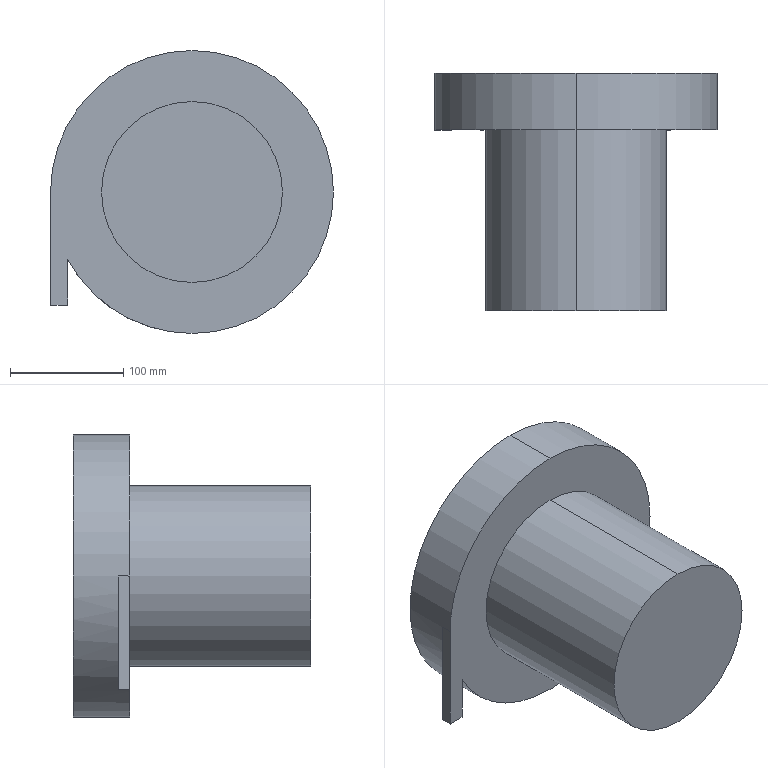Part | STEP file | Vibration plate3 | 1 solid | 11 faces | box 250 x 210 x 250 mm | volume 5680348 mm3 | plane 7 | cylinder 4 | commonest cylinder face diameters 160 x2 250 x2
STEP:
#1=CARTESIAN_POINT('',(0.,0.,0.));
#2=DIRECTION('',(0.,0.,1.));
#3=DIRECTION('',(1.,0.,0.));
#4=AXIS2_PLACEMENT_3D('',#1,#2,#3);
#5=CARTESIAN_POINT('',(0.,210.,125.));
#6=VERTEX_POINT('',#5);
#7=CARTESIAN_POINT('',(0.,210.,-125.));
#8=VERTEX_POINT('',#7);
#9=CARTESIAN_POINT('',(0.,210.,0.));
#10=DIRECTION('',(0.,1.,0.));
#11=DIRECTION('',(0.,0.,1.));
#12=AXIS2_PLACEMENT_3D('',#9,#10,#11);
#13=CIRCLE('',#12,125.);
#14=CARTESIAN_POINT('',(0.,210.,0.));
#15=DIRECTION('',(0.,-1.,0.));
#16=DIRECTION('',(0.,0.,-1.));
#17=AXIS2_PLACEMENT_3D('',#14,#15,#16);
#18=CYLINDRICAL_SURFACE('',#17,125.);
#19=CARTESIAN_POINT('',(3.142,0.));
#20=DIRECTION('',(-1.,0.));
#21=VECTOR('',#20,1.);
#22=LINE('',#19,#21);
#23=(GEOMETRIC_REPRESENTATION_CONTEXT(2)PARAMETRIC_REPRESENTATION_CONTEXT()REPRESENTATION_CONTEXT('',''));
#24=DEFINITIONAL_REPRESENTATION('',(#22),#23);
#25=PCURVE('',#18,#24);
#26=CARTESIAN_POINT('',(0.,210.,0.));
#27=DIRECTION('',(0.,1.,0.));
#28=DIRECTION('',(0.,0.,1.));
#29=AXIS2_PLACEMENT_3D('',#26,#27,#28);
#30=PLANE('',#29);
#31=CARTESIAN_POINT('',(0.,0.));
#32=DIRECTION('',(1.,0.));
#33=AXIS2_PLACEMENT_2D('',#31,#32);
#34=CIRCLE('',#33,125.);
#35=(GEOMETRIC_REPRESENTATION_CONTEXT(2)PARAMETRIC_REPRESENTATION_CONTEXT()REPRESENTATION_CONTEXT('',''));
#36=DEFINITIONAL_REPRESENTATION('',(#34),#35);
#37=PCURVE('',#30,#36);
#38=SURFACE_CURVE('',#13,(#25,#37),.PCURVE_S1.);
#39=EDGE_CURVE('',#6,#8,#38,.T.);
#40=ORIENTED_EDGE('',*,*,#39,.F.);
#41=CARTESIAN_POINT('',(0.,160.,125.));
#42=VERTEX_POINT('',#41);
#43=CARTESIAN_POINT('',(0.,210.,125.));
#44=DIRECTION('',(0.,-1.,0.));
#45=VECTOR('',#44,1.);
#46=LINE('',#43,#45);
#47=CARTESIAN_POINT('',(3.142,0.));
#48=DIRECTION('',(0.,1.));
#49=VECTOR('',#48,1.);
#50=LINE('',#47,#49);
#51=(GEOMETRIC_REPRESENTATION_CONTEXT(2)PARAMETRIC_REPRESENTATION_CONTEXT()REPRESENTATION_CONTEXT('',''));
#52=DEFINITIONAL_REPRESENTATION('',(#50),#51);
#53=PCURVE('',#18,#52);
#54=CARTESIAN_POINT('',(0.,210.,0.));
#55=DIRECTION('',(0.,-1.,0.));
#56=DIRECTION('',(0.,0.,-1.));
#57=AXIS2_PLACEMENT_3D('',#54,#55,#56);
#58=CYLINDRICAL_SURFACE('',#57,125.);
#59=CARTESIAN_POINT('',(3.142,0.));
#60=DIRECTION('',(0.,1.));
#61=VECTOR('',#60,1.);
#62=LINE('',#59,#61);
#63=(GEOMETRIC_REPRESENTATION_CONTEXT(2)PARAMETRIC_REPRESENTATION_CONTEXT()REPRESENTATION_CONTEXT('',''));
#64=DEFINITIONAL_REPRESENTATION('',(#62),#63);
#65=PCURVE('',#58,#64);
#66=SURFACE_CURVE('',#46,(#53,#65),.PCURVE_S1.);
#67=EDGE_CURVE('',#6,#42,#66,.T.);
#68=ORIENTED_EDGE('',*,*,#67,.T.);
#69=CARTESIAN_POINT('',(0.,160.,-125.));
#70=VERTEX_POINT('',#69);
#71=CARTESIAN_POINT('',(0.,160.,0.));
#72=DIRECTION('',(0.,1.,0.));
#73=DIRECTION('',(0.,0.,1.));
#74=AXIS2_PLACEMENT_3D('',#71,#72,#73);
#75=CIRCLE('',#74,125.);
#76=CARTESIAN_POINT('',(3.142,50.));
#77=DIRECTION('',(-1.,0.));
#78=VECTOR('',#77,1.);
#79=LINE('',#76,#78);
#80=(GEOMETRIC_REPRESENTATION_CONTEXT(2)PARAMETRIC_REPRESENTATION_CONTEXT()REPRESENTATION_CONTEXT('',''));
#81=DEFINITIONAL_REPRESENTATION('',(#79),#80);
#82=PCURVE('',#18,#81);
#83=CARTESIAN_POINT('',(0.,160.,0.));
#84=DIRECTION('',(0.,1.,0.));
#85=DIRECTION('',(0.,0.,1.));
#86=AXIS2_PLACEMENT_3D('',#83,#84,#85);
#87=PLANE('',#86);
#88=CARTESIAN_POINT('',(0.,0.));
#89=DIRECTION('',(1.,0.));
#90=AXIS2_PLACEMENT_2D('',#88,#89);
#91=CIRCLE('',#90,125.);
#92=(GEOMETRIC_REPRESENTATION_CONTEXT(2)PARAMETRIC_REPRESENTATION_CONTEXT()REPRESENTATION_CONTEXT('',''));
#93=DEFINITIONAL_REPRESENTATION('',(#91),#92);
#94=PCURVE('',#87,#93);
#95=SURFACE_CURVE('',#75,(#82,#94),.PCURVE_S1.);
#96=EDGE_CURVE('',#42,#70,#95,.T.);
#97=ORIENTED_EDGE('',*,*,#96,.T.);
#98=CARTESIAN_POINT('',(0.,210.,-125.));
#99=DIRECTION('',(0.,-1.,0.));
#100=VECTOR('',#99,1.);
#101=LINE('',#98,#100);
#102=CARTESIAN_POINT('',(0.,0.));
#103=DIRECTION('',(0.,1.));
#104=VECTOR('',#103,1.);
#105=LINE('',#102,#104);
#106=(GEOMETRIC_REPRESENTATION_CONTEXT(2)PARAMETRIC_REPRESENTATION_CONTEXT()REPRESENTATION_CONTEXT('',''));
#107=DEFINITIONAL_REPRESENTATION('',(#105),#106);
#108=PCURVE('',#18,#107);
#109=CARTESIAN_POINT('',(6.283,0.));
#110=DIRECTION('',(0.,1.));
#111=VECTOR('',#110,1.);
#112=LINE('',#109,#111);
#113=(GEOMETRIC_REPRESENTATION_CONTEXT(2)PARAMETRIC_REPRESENTATION_CONTEXT()REPRESENTATION_CONTEXT('',''));
#114=DEFINITIONAL_REPRESENTATION('',(#112),#113);
#115=PCURVE('',#58,#114);
#116=SURFACE_CURVE('',#101,(#108,#115),.PCURVE_S1.);
#117=EDGE_CURVE('',#8,#70,#116,.T.);
#118=ORIENTED_EDGE('',*,*,#117,.F.);
#119=EDGE_LOOP('',(#40,#68,#97,#118));
#120=FACE_BOUND('',#119,.T.);
#121=ADVANCED_FACE('',(#120),#18,.T.);
#122=CARTESIAN_POINT('',(0.,160.,80.));
#123=VERTEX_POINT('',#122);
#124=CARTESIAN_POINT('',(0.,160.,-80.));
#125=VERTEX_POINT('',#124);
#126=CARTESIAN_POINT('',(0.,160.,0.));
#127=DIRECTION('',(0.,1.,0.));
#128=DIRECTION('',(0.,0.,1.));
#129=AXIS2_PLACEMENT_3D('',#126,#127,#128);
#130=CIRCLE('',#129,80.);
#131=CARTESIAN_POINT('',(0.,160.,0.));
#132=DIRECTION('',(0.,-1.,0.));
#133=DIRECTION('',(0.,0.,-1.));
#134=AXIS2_PLACEMENT_3D('',#131,#132,#133);
#135=CYLINDRICAL_SURFACE('',#134,80.);
#136=CARTESIAN_POINT('',(3.142,0.));
#137=DIRECTION('',(-1.,0.));
#138=VECTOR('',#137,1.);
#139=LINE('',#136,#138);
#140=(GEOMETRIC_REPRESENTATION_CONTEXT(2)PARAMETRIC_REPRESENTATION_CONTEXT()REPRESENTATION_CONTEXT('',''));
#141=DEFINITIONAL_REPRESENTATION('',(#139),#140);
#142=PCURVE('',#135,#141);
#143=CARTESIAN_POINT('',(0.,0.));
#144=DIRECTION('',(1.,0.));
#145=AXIS2_PLACEMENT_2D('',#143,#144);
#146=CIRCLE('',#145,80.);
#147=(GEOMETRIC_REPRESENTATION_CONTEXT(2)PARAMETRIC_REPRESENTATION_CONTEXT()REPRESENTATION_CONTEXT('',''));
#148=DEFINITIONAL_REPRESENTATION('',(#146),#147);
#149=PCURVE('',#87,#148);
#150=SURFACE_CURVE('',#130,(#142,#149),.PCURVE_S1.);
#151=EDGE_CURVE('',#123,#125,#150,.T.);
#152=ORIENTED_EDGE('',*,*,#151,.F.);
#153=CARTESIAN_POINT('',(0.,0.,80.));
#154=VERTEX_POINT('',#153);
#155=CARTESIAN_POINT('',(0.,160.,80.));
#156=DIRECTION('',(0.,-1.,0.));
#157=VECTOR('',#156,1.);
#158=LINE('',#155,#157);
#159=CARTESIAN_POINT('',(3.142,0.));
#160=DIRECTION('',(0.,1.));
#161=VECTOR('',#160,1.);
#162=LINE('',#159,#161);
#163=(GEOMETRIC_REPRESENTATION_CONTEXT(2)PARAMETRIC_REPRESENTATION_CONTEXT()REPRESENTATION_CONTEXT('',''));
#164=DEFINITIONAL_REPRESENTATION('',(#162),#163);
#165=PCURVE('',#135,#164);
#166=CARTESIAN_POINT('',(0.,160.,0.));
#167=DIRECTION('',(0.,-1.,0.));
#168=DIRECTION('',(0.,0.,-1.));
#169=AXIS2_PLACEMENT_3D('',#166,#167,#168);
#170=CYLINDRICAL_SURFACE('',#169,80.);
#171=CARTESIAN_POINT('',(3.142,0.));
#172=DIRECTION('',(0.,1.));
#173=VECTOR('',#172,1.);
#174=LINE('',#171,#173);
#175=(GEOMETRIC_REPRESENTATION_CONTEXT(2)PARAMETRIC_REPRESENTATION_CONTEXT()REPRESENTATION_CONTEXT('',''));
#176=DEFINITIONAL_REPRESENTATION('',(#174),#175);
#177=PCURVE('',#170,#176);
#178=SURFACE_CURVE('',#158,(#165,#177),.PCURVE_S1.);
#179=EDGE_CURVE('',#123,#154,#178,.T.);
#180=ORIENTED_EDGE('',*,*,#179,.T.);
#181=CARTESIAN_POINT('',(0.,0.,-80.));
#182=VERTEX_POINT('',#181);
#183=CARTESIAN_POINT('',(0.,0.,0.));
#184=DIRECTION('',(0.,1.,0.));
#185=DIRECTION('',(0.,0.,1.));
#186=AXIS2_PLACEMENT_3D('',#183,#184,#185);
#187=CIRCLE('',#186,80.);
#188=CARTESIAN_POINT('',(3.142,160.));
#189=DIRECTION('',(-1.,0.));
#190=VECTOR('',#189,1.);
#191=LINE('',#188,#190);
#192=(GEOMETRIC_REPRESENTATION_CONTEXT(2)PARAMETRIC_REPRESENTATION_CONTEXT()REPRESENTATION_CONTEXT('',''));
#193=DEFINITIONAL_REPRESENTATION('',(#191),#192);
#194=PCURVE('',#135,#193);
#195=CARTESIAN_POINT('',(0.,0.,0.));
#196=DIRECTION('',(0.,1.,0.));
#197=DIRECTION('',(0.,0.,1.));
#198=AXIS2_PLACEMENT_3D('',#195,#196,#197);
#199=PLANE('',#198);
#200=CARTESIAN_POINT('',(0.,0.));
#201=DIRECTION('',(1.,0.));
#202=AXIS2_PLACEMENT_2D('',#200,#201);
#203=CIRCLE('',#202,80.);
#204=(GEOMETRIC_REPRESENTATION_CONTEXT(2)PARAMETRIC_REPRESENTATION_CONTEXT()REPRESENTATION_CONTEXT('',''));
#205=DEFINITIONAL_REPRESENTATION('',(#203),#204);
#206=PCURVE('',#199,#205);
#207=SURFACE_CURVE('',#187,(#194,#206),.PCURVE_S1.);
#208=EDGE_CURVE('',#154,#182,#207,.T.);
#209=ORIENTED_EDGE('',*,*,#208,.T.);
#210=CARTESIAN_POINT('',(0.,160.,-80.));
#211=DIRECTION('',(0.,-1.,0.));
#212=VECTOR('',#211,1.);
#213=LINE('',#210,#212);
#214=CARTESIAN_POINT('',(0.,0.));
#215=DIRECTION('',(0.,1.));
#216=VECTOR('',#215,1.);
#217=LINE('',#214,#216);
#218=(GEOMETRIC_REPRESENTATION_CONTEXT(2)PARAMETRIC_REPRESENTATION_CONTEXT()REPRESENTATION_CONTEXT('',''));
#219=DEFINITIONAL_REPRESENTATION('',(#217),#218);
#220=PCURVE('',#135,#219);
#221=CARTESIAN_POINT('',(6.283,0.));
#222=DIRECTION('',(0.,1.));
#223=VECTOR('',#222,1.);
#224=LINE('',#221,#223);
#225=(GEOMETRIC_REPRESENTATION_CONTEXT(2)PARAMETRIC_REPRESENTATION_CONTEXT()REPRESENTATION_CONTEXT('',''));
#226=DEFINITIONAL_REPRESENTATION('',(#224),#225);
#227=PCURVE('',#170,#226);
#228=SURFACE_CURVE('',#213,(#220,#227),.PCURVE_S1.);
#229=EDGE_CURVE('',#125,#182,#228,.T.);
#230=ORIENTED_EDGE('',*,*,#229,.F.);
#231=EDGE_LOOP('',(#152,#180,#209,#230));
#232=FACE_BOUND('',#231,.T.);
#233=ADVANCED_FACE('',(#232),#135,.T.);
#234=ORIENTED_EDGE('',*,*,#179,.F.);
#235=CARTESIAN_POINT('',(0.,160.,0.));
#236=DIRECTION('',(0.,1.,0.));
#237=DIRECTION('',(0.,0.,1.));
#238=AXIS2_PLACEMENT_3D('',#235,#236,#237);
#239=CIRCLE('',#238,80.);
#240=CARTESIAN_POINT('',(9.425,0.));
#241=DIRECTION('',(-1.,0.));
#242=VECTOR('',#241,1.);
#243=LINE('',#240,#242);
#244=(GEOMETRIC_REPRESENTATION_CONTEXT(2)PARAMETRIC_REPRESENTATION_CONTEXT()REPRESENTATION_CONTEXT('',''));
#245=DEFINITIONAL_REPRESENTATION('',(#243),#244);
#246=PCURVE('',#170,#245);
#247=CARTESIAN_POINT('',(0.,0.));
#248=DIRECTION('',(1.,0.));
#249=AXIS2_PLACEMENT_2D('',#247,#248);
#250=CIRCLE('',#249,80.);
#251=(GEOMETRIC_REPRESENTATION_CONTEXT(2)PARAMETRIC_REPRESENTATION_CONTEXT()REPRESENTATION_CONTEXT('',''));
#252=DEFINITIONAL_REPRESENTATION('',(#250),#251);
#253=PCURVE('',#87,#252);
#254=SURFACE_CURVE('',#239,(#246,#253),.PCURVE_S1.);
#255=EDGE_CURVE('',#125,#123,#254,.T.);
#256=ORIENTED_EDGE('',*,*,#255,.F.);
#257=ORIENTED_EDGE('',*,*,#229,.T.);
#258=CARTESIAN_POINT('',(0.,0.,0.));
#259=DIRECTION('',(0.,1.,0.));
#260=DIRECTION('',(0.,0.,1.));
#261=AXIS2_PLACEMENT_3D('',#258,#259,#260);
#262=CIRCLE('',#261,80.);
#263=CARTESIAN_POINT('',(9.425,160.));
#264=DIRECTION('',(-1.,0.));
#265=VECTOR('',#264,1.);
#266=LINE('',#263,#265);
#267=(GEOMETRIC_REPRESENTATION_CONTEXT(2)PARAMETRIC_REPRESENTATION_CONTEXT()REPRESENTATION_CONTEXT('',''));
#268=DEFINITIONAL_REPRESENTATION('',(#266),#267);
#269=PCURVE('',#170,#268);
#270=CARTESIAN_POINT('',(0.,0.));
#271=DIRECTION('',(1.,0.));
#272=AXIS2_PLACEMENT_2D('',#270,#271);
#273=CIRCLE('',#272,80.);
#274=(GEOMETRIC_REPRESENTATION_CONTEXT(2)PARAMETRIC_REPRESENTATION_CONTEXT()REPRESENTATION_CONTEXT('',''));
#275=DEFINITIONAL_REPRESENTATION('',(#273),#274);
#276=PCURVE('',#199,#275);
#277=SURFACE_CURVE('',#262,(#269,#276),.PCURVE_S1.);
#278=EDGE_CURVE('',#182,#154,#277,.T.);
#279=ORIENTED_EDGE('',*,*,#278,.T.);
#280=EDGE_LOOP('',(#234,#256,#257,#279));
#281=FACE_BOUND('',#280,.T.);
#282=ADVANCED_FACE('',(#281),#170,.T.);
#283=ORIENTED_EDGE('',*,*,#278,.F.);
#284=ORIENTED_EDGE('',*,*,#208,.F.);
#285=EDGE_LOOP('',(#283,#284));
#286=FACE_BOUND('',#285,.T.);
#287=ADVANCED_FACE('',(#286),#199,.F.);
#288=CARTESIAN_POINT('',(-125.,160.,0.));
#289=VERTEX_POINT('',#288);
#290=CARTESIAN_POINT('',(0.,160.,0.));
#291=DIRECTION('',(0.,1.,0.));
#292=DIRECTION('',(0.,0.,1.));
#293=AXIS2_PLACEMENT_3D('',#290,#291,#292);
#294=CIRCLE('',#293,125.);
#295=CARTESIAN_POINT('',(0.,0.));
#296=DIRECTION('',(1.,0.));
#297=AXIS2_PLACEMENT_2D('',#295,#296);
#298=CIRCLE('',#297,125.);
#299=(GEOMETRIC_REPRESENTATION_CONTEXT(2)PARAMETRIC_REPRESENTATION_CONTEXT()REPRESENTATION_CONTEXT('',''));
#300=DEFINITIONAL_REPRESENTATION('',(#298),#299);
#301=PCURVE('',#87,#300);
#302=CARTESIAN_POINT('',(9.425,50.));
#303=DIRECTION('',(-1.,0.));
#304=VECTOR('',#303,1.);
#305=LINE('',#302,#304);
#306=(GEOMETRIC_REPRESENTATION_CONTEXT(2)PARAMETRIC_REPRESENTATION_CONTEXT()REPRESENTATION_CONTEXT('',''));
#307=DEFINITIONAL_REPRESENTATION('',(#305),#306);
#308=PCURVE('',#58,#307);
#309=SURFACE_CURVE('',#294,(#301,#308),.PCURVE_S1.);
#310=EDGE_CURVE('',#289,#42,#309,.T.);
#311=ORIENTED_EDGE('',*,*,#310,.F.);
#312=CARTESIAN_POINT('',(-125.,160.,-100.));
#313=VERTEX_POINT('',#312);
#314=CARTESIAN_POINT('',(-125.,160.,0.));
#315=DIRECTION('',(0.,0.,-1.));
#316=VECTOR('',#315,1.);
#317=LINE('',#314,#316);
#318=CARTESIAN_POINT('',(0.,-125.));
#319=DIRECTION('',(-1.,0.));
#320=VECTOR('',#319,1.);
#321=LINE('',#318,#320);
#322=(GEOMETRIC_REPRESENTATION_CONTEXT(2)PARAMETRIC_REPRESENTATION_CONTEXT()REPRESENTATION_CONTEXT('',''));
#323=DEFINITIONAL_REPRESENTATION('',(#321),#322);
#324=PCURVE('',#87,#323);
#325=CARTESIAN_POINT('',(-125.,170.,0.));
#326=DIRECTION('',(-1.,0.,0.));
#327=DIRECTION('',(0.,0.,1.));
#328=AXIS2_PLACEMENT_3D('',#325,#326,#327);
#329=PLANE('',#328);
#330=CARTESIAN_POINT('',(0.,-10.));
#331=DIRECTION('',(-1.,0.));
#332=VECTOR('',#331,1.);
#333=LINE('',#330,#332);
#334=(GEOMETRIC_REPRESENTATION_CONTEXT(2)PARAMETRIC_REPRESENTATION_CONTEXT()REPRESENTATION_CONTEXT('',''));
#335=DEFINITIONAL_REPRESENTATION('',(#333),#334);
#336=PCURVE('',#329,#335);
#337=SURFACE_CURVE('',#317,(#324,#336),.PCURVE_S1.);
#338=EDGE_CURVE('',#289,#313,#337,.T.);
#339=ORIENTED_EDGE('',*,*,#338,.T.);
#340=CARTESIAN_POINT('',(-110.,160.,-100.));
#341=VERTEX_POINT('',#340);
#342=CARTESIAN_POINT('',(-125.,160.,-100.));
#343=DIRECTION('',(1.,0.,0.));
#344=VECTOR('',#343,1.);
#345=LINE('',#342,#344);
#346=CARTESIAN_POINT('',(-100.,-125.));
#347=DIRECTION('',(0.,1.));
#348=VECTOR('',#347,1.);
#349=LINE('',#346,#348);
#350=(GEOMETRIC_REPRESENTATION_CONTEXT(2)PARAMETRIC_REPRESENTATION_CONTEXT()REPRESENTATION_CONTEXT('',''));
#351=DEFINITIONAL_REPRESENTATION('',(#349),#350);
#352=PCURVE('',#87,#351);
#353=CARTESIAN_POINT('',(-125.,170.,-100.));
#354=DIRECTION('',(0.,0.,-1.));
#355=DIRECTION('',(-1.,0.,0.));
#356=AXIS2_PLACEMENT_3D('',#353,#354,#355);
#357=PLANE('',#356);
#358=CARTESIAN_POINT('',(0.,-10.));
#359=DIRECTION('',(-1.,0.));
#360=VECTOR('',#359,1.);
#361=LINE('',#358,#360);
#362=(GEOMETRIC_REPRESENTATION_CONTEXT(2)PARAMETRIC_REPRESENTATION_CONTEXT()REPRESENTATION_CONTEXT('',''));
#363=DEFINITIONAL_REPRESENTATION('',(#361),#362);
#364=PCURVE('',#357,#363);
#365=SURFACE_CURVE('',#345,(#352,#364),.PCURVE_S1.);
#366=EDGE_CURVE('',#313,#341,#365,.T.);
#367=ORIENTED_EDGE('',*,*,#366,.T.);
#368=CARTESIAN_POINT('',(-110.,160.,-59.372));
#369=VERTEX_POINT('',#368);
#370=CARTESIAN_POINT('',(-110.,160.,0.));
#371=DIRECTION('',(0.,0.,1.));
#372=VECTOR('',#371,1.);
#373=LINE('',#370,#372);
#374=CARTESIAN_POINT('',(0.,-110.));
#375=DIRECTION('',(1.,0.));
#376=VECTOR('',#375,1.);
#377=LINE('',#374,#376);
#378=(GEOMETRIC_REPRESENTATION_CONTEXT(2)PARAMETRIC_REPRESENTATION_CONTEXT()REPRESENTATION_CONTEXT('',''));
#379=DEFINITIONAL_REPRESENTATION('',(#377),#378);
#380=PCURVE('',#87,#379);
#381=CARTESIAN_POINT('',(-110.,170.,0.));
#382=DIRECTION('',(1.,0.,0.));
#383=DIRECTION('',(0.,0.,-1.));
#384=AXIS2_PLACEMENT_3D('',#381,#382,#383);
#385=PLANE('',#384);
#386=CARTESIAN_POINT('',(0.,-10.));
#387=DIRECTION('',(-1.,0.));
#388=VECTOR('',#387,1.);
#389=LINE('',#386,#388);
#390=(GEOMETRIC_REPRESENTATION_CONTEXT(2)PARAMETRIC_REPRESENTATION_CONTEXT()REPRESENTATION_CONTEXT('',''));
#391=DEFINITIONAL_REPRESENTATION('',(#389),#390);
#392=PCURVE('',#385,#391);
#393=SURFACE_CURVE('',#373,(#380,#392),.PCURVE_S1.);
#394=EDGE_CURVE('',#341,#369,#393,.T.);
#395=ORIENTED_EDGE('',*,*,#394,.T.);
#396=CARTESIAN_POINT('',(0.,160.,0.));
#397=DIRECTION('',(0.,1.,0.));
#398=DIRECTION('',(0.,0.,1.));
#399=AXIS2_PLACEMENT_3D('',#396,#397,#398);
#400=CIRCLE('',#399,125.);
#401=CARTESIAN_POINT('',(0.,0.));
#402=DIRECTION('',(1.,0.));
#403=AXIS2_PLACEMENT_2D('',#401,#402);
#404=CIRCLE('',#403,125.);
#405=(GEOMETRIC_REPRESENTATION_CONTEXT(2)PARAMETRIC_REPRESENTATION_CONTEXT()REPRESENTATION_CONTEXT('',''));
#406=DEFINITIONAL_REPRESENTATION('',(#404),#405);
#407=PCURVE('',#87,#406);
#408=CARTESIAN_POINT('',(9.425,50.));
#409=DIRECTION('',(-1.,0.));
#410=VECTOR('',#409,1.);
#411=LINE('',#408,#410);
#412=(GEOMETRIC_REPRESENTATION_CONTEXT(2)PARAMETRIC_REPRESENTATION_CONTEXT()REPRESENTATION_CONTEXT('',''));
#413=DEFINITIONAL_REPRESENTATION('',(#411),#412);
#414=PCURVE('',#58,#413);
#415=SURFACE_CURVE('',#400,(#407,#414),.PCURVE_S1.);
#416=EDGE_CURVE('',#70,#369,#415,.T.);
#417=ORIENTED_EDGE('',*,*,#416,.F.);
#418=ORIENTED_EDGE('',*,*,#96,.F.);
#419=EDGE_LOOP('',(#311,#339,#367,#395,#417,#418));
#420=FACE_BOUND('',#419,.T.);
#421=ORIENTED_EDGE('',*,*,#255,.T.);
#422=ORIENTED_EDGE('',*,*,#151,.T.);
#423=EDGE_LOOP('',(#421,#422));
#424=FACE_BOUND('',#423,.T.);
#425=ADVANCED_FACE('',(#420,#424),#87,.F.);
#426=ORIENTED_EDGE('',*,*,#67,.F.);
#427=CARTESIAN_POINT('',(0.,210.,0.));
#428=DIRECTION('',(0.,1.,0.));
#429=DIRECTION('',(0.,0.,1.));
#430=AXIS2_PLACEMENT_3D('',#427,#428,#429);
#431=CIRCLE('',#430,125.);
#432=CARTESIAN_POINT('',(9.425,0.));
#433=DIRECTION('',(-1.,0.));
#434=VECTOR('',#433,1.);
#435=LINE('',#432,#434);
#436=(GEOMETRIC_REPRESENTATION_CONTEXT(2)PARAMETRIC_REPRESENTATION_CONTEXT()REPRESENTATION_CONTEXT('',''));
#437=DEFINITIONAL_REPRESENTATION('',(#435),#436);
#438=PCURVE('',#58,#437);
#439=CARTESIAN_POINT('',(0.,0.));
#440=DIRECTION('',(1.,0.));
#441=AXIS2_PLACEMENT_2D('',#439,#440);
#442=CIRCLE('',#441,125.);
#443=(GEOMETRIC_REPRESENTATION_CONTEXT(2)PARAMETRIC_REPRESENTATION_CONTEXT()REPRESENTATION_CONTEXT('',''));
#444=DEFINITIONAL_REPRESENTATION('',(#442),#443);
#445=PCURVE('',#30,#444);
#446=SURFACE_CURVE('',#431,(#438,#445),.PCURVE_S1.);
#447=EDGE_CURVE('',#8,#6,#446,.T.);
#448=ORIENTED_EDGE('',*,*,#447,.F.);
#449=ORIENTED_EDGE('',*,*,#117,.T.);
#450=ORIENTED_EDGE('',*,*,#416,.T.);
#451=CARTESIAN_POINT('',(-110.,170.,-59.372));
#452=VERTEX_POINT('',#451);
#453=CARTESIAN_POINT('',(-110.,210.,-59.372));
#454=DIRECTION('',(0.,1.,0.));
#455=VECTOR('',#454,1.);
#456=LINE('',#453,#455);
#457=CARTESIAN_POINT('',(5.207,0.));
#458=DIRECTION('',(0.,-1.));
#459=VECTOR('',#458,1.);
#460=LINE('',#457,#459);
#461=(GEOMETRIC_REPRESENTATION_CONTEXT(2)PARAMETRIC_REPRESENTATION_CONTEXT()REPRESENTATION_CONTEXT('',''));
#462=DEFINITIONAL_REPRESENTATION('',(#460),#461);
#463=PCURVE('',#58,#462);
#464=CARTESIAN_POINT('',(59.372,40.));
#465=DIRECTION('',(0.,1.));
#466=VECTOR('',#465,1.);
#467=LINE('',#464,#466);
#468=(GEOMETRIC_REPRESENTATION_CONTEXT(2)PARAMETRIC_REPRESENTATION_CONTEXT()REPRESENTATION_CONTEXT('',''));
#469=DEFINITIONAL_REPRESENTATION('',(#467),#468);
#470=PCURVE('',#385,#469);
#471=SURFACE_CURVE('',#456,(#463,#470),.PCURVE_S1.);
#472=EDGE_CURVE('',#369,#452,#471,.T.);
#473=ORIENTED_EDGE('',*,*,#472,.T.);
#474=CARTESIAN_POINT('',(-125.,170.,0.));
#475=VERTEX_POINT('',#474);
#476=CARTESIAN_POINT('',(0.,170.,0.));
#477=DIRECTION('',(0.,-1.,0.));
#478=DIRECTION('',(0.,0.,-1.));
#479=AXIS2_PLACEMENT_3D('',#476,#477,#478);
#480=CIRCLE('',#479,125.);
#481=CARTESIAN_POINT('',(0.,40.));
#482=DIRECTION('',(1.,0.));
#483=VECTOR('',#482,1.);
#484=LINE('',#481,#483);
#485=(GEOMETRIC_REPRESENTATION_CONTEXT(2)PARAMETRIC_REPRESENTATION_CONTEXT()REPRESENTATION_CONTEXT('',''));
#486=DEFINITIONAL_REPRESENTATION('',(#484),#485);
#487=PCURVE('',#58,#486);
#488=CARTESIAN_POINT('',(0.,170.,0.));
#489=DIRECTION('',(0.,-1.,0.));
#490=DIRECTION('',(0.,0.,-1.));
#491=AXIS2_PLACEMENT_3D('',#488,#489,#490);
#492=PLANE('',#491);
#493=CARTESIAN_POINT('',(0.,0.));
#494=DIRECTION('',(1.,0.));
#495=AXIS2_PLACEMENT_2D('',#493,#494);
#496=CIRCLE('',#495,125.);
#497=(GEOMETRIC_REPRESENTATION_CONTEXT(2)PARAMETRIC_REPRESENTATION_CONTEXT()REPRESENTATION_CONTEXT('',''));
#498=DEFINITIONAL_REPRESENTATION('',(#496),#497);
#499=PCURVE('',#492,#498);
#500=SURFACE_CURVE('',#480,(#487,#499),.PCURVE_S1.);
#501=EDGE_CURVE('',#475,#452,#500,.T.);
#502=ORIENTED_EDGE('',*,*,#501,.F.);
#503=CARTESIAN_POINT('',(-125.,170.,0.));
#504=DIRECTION('',(0.,-1.,0.));
#505=VECTOR('',#504,1.);
#506=LINE('',#503,#505);
#507=CARTESIAN_POINT('',(4.712,40.));
#508=DIRECTION('',(0.,1.));
#509=VECTOR('',#508,1.);
#510=LINE('',#507,#509);
#511=(GEOMETRIC_REPRESENTATION_CONTEXT(2)PARAMETRIC_REPRESENTATION_CONTEXT()REPRESENTATION_CONTEXT('',''));
#512=DEFINITIONAL_REPRESENTATION('',(#510),#511);
#513=PCURVE('',#58,#512);
#514=CARTESIAN_POINT('',(0.,0.));
#515=DIRECTION('',(0.,-1.));
#516=VECTOR('',#515,1.);
#517=LINE('',#514,#516);
#518=(GEOMETRIC_REPRESENTATION_CONTEXT(2)PARAMETRIC_REPRESENTATION_CONTEXT()REPRESENTATION_CONTEXT('',''));
#519=DEFINITIONAL_REPRESENTATION('',(#517),#518);
#520=PCURVE('',#329,#519);
#521=SURFACE_CURVE('',#506,(#513,#520),.PCURVE_S1.);
#522=EDGE_CURVE('',#475,#289,#521,.T.);
#523=ORIENTED_EDGE('',*,*,#522,.T.);
#524=ORIENTED_EDGE('',*,*,#310,.T.);
#525=EDGE_LOOP('',(#426,#448,#449,#450,#473,#502,#523,#524));
#526=FACE_BOUND('',#525,.T.);
#527=ADVANCED_FACE('',(#526),#58,.T.);
#528=ORIENTED_EDGE('',*,*,#447,.T.);
#529=ORIENTED_EDGE('',*,*,#39,.T.);
#530=EDGE_LOOP('',(#528,#529));
#531=FACE_BOUND('',#530,.T.);
#532=ADVANCED_FACE('',(#531),#30,.T.);
#533=ORIENTED_EDGE('',*,*,#472,.F.);
#534=ORIENTED_EDGE('',*,*,#394,.F.);
#535=CARTESIAN_POINT('',(-110.,170.,-100.));
#536=VERTEX_POINT('',#535);
#537=CARTESIAN_POINT('',(-110.,170.,-100.));
#538=DIRECTION('',(0.,-1.,0.));
#539=VECTOR('',#538,1.);
#540=LINE('',#537,#539);
#541=CARTESIAN_POINT('',(100.,0.));
#542=DIRECTION('',(0.,-1.));
#543=VECTOR('',#542,1.);
#544=LINE('',#541,#543);
#545=(GEOMETRIC_REPRESENTATION_CONTEXT(2)PARAMETRIC_REPRESENTATION_CONTEXT()REPRESENTATION_CONTEXT('',''));
#546=DEFINITIONAL_REPRESENTATION('',(#544),#545);
#547=PCURVE('',#385,#546);
#548=CARTESIAN_POINT('',(-15.,0.));
#549=DIRECTION('',(0.,-1.));
#550=VECTOR('',#549,1.);
#551=LINE('',#548,#550);
#552=(GEOMETRIC_REPRESENTATION_CONTEXT(2)PARAMETRIC_REPRESENTATION_CONTEXT()REPRESENTATION_CONTEXT('',''));
#553=DEFINITIONAL_REPRESENTATION('',(#551),#552);
#554=PCURVE('',#357,#553);
#555=SURFACE_CURVE('',#540,(#547,#554),.PCURVE_S1.);
#556=EDGE_CURVE('',#536,#341,#555,.T.);
#557=ORIENTED_EDGE('',*,*,#556,.F.);
#558=CARTESIAN_POINT('',(-110.,170.,0.));
#559=DIRECTION('',(0.,0.,1.));
#560=VECTOR('',#559,1.);
#561=LINE('',#558,#560);
#562=CARTESIAN_POINT('',(0.,0.));
#563=DIRECTION('',(-1.,0.));
#564=VECTOR('',#563,1.);
#565=LINE('',#562,#564);
#566=(GEOMETRIC_REPRESENTATION_CONTEXT(2)PARAMETRIC_REPRESENTATION_CONTEXT()REPRESENTATION_CONTEXT('',''));
#567=DEFINITIONAL_REPRESENTATION('',(#565),#566);
#568=PCURVE('',#385,#567);
#569=CARTESIAN_POINT('',(0.,-110.));
#570=DIRECTION('',(-1.,0.));
#571=VECTOR('',#570,1.);
#572=LINE('',#569,#571);
#573=(GEOMETRIC_REPRESENTATION_CONTEXT(2)PARAMETRIC_REPRESENTATION_CONTEXT()REPRESENTATION_CONTEXT('',''));
#574=DEFINITIONAL_REPRESENTATION('',(#572),#573);
#575=PCURVE('',#492,#574);
#576=SURFACE_CURVE('',#561,(#568,#575),.PCURVE_S1.);
#577=EDGE_CURVE('',#536,#452,#576,.T.);
#578=ORIENTED_EDGE('',*,*,#577,.T.);
#579=EDGE_LOOP('',(#533,#534,#557,#578));
#580=FACE_BOUND('',#579,.T.);
#581=ADVANCED_FACE('',(#580),#385,.T.);
#582=CARTESIAN_POINT('',(-125.,170.,-100.));
#583=VERTEX_POINT('',#582);
#584=CARTESIAN_POINT('',(-125.,170.,0.));
#585=DIRECTION('',(0.,0.,-1.));
#586=VECTOR('',#585,1.);
#587=LINE('',#584,#586);
#588=CARTESIAN_POINT('',(0.,-125.));
#589=DIRECTION('',(1.,0.));
#590=VECTOR('',#589,1.);
#591=LINE('',#588,#590);
#592=(GEOMETRIC_REPRESENTATION_CONTEXT(2)PARAMETRIC_REPRESENTATION_CONTEXT()REPRESENTATION_CONTEXT('',''));
#593=DEFINITIONAL_REPRESENTATION('',(#591),#592);
#594=PCURVE('',#492,#593);
#595=CARTESIAN_POINT('',(0.,0.));
#596=DIRECTION('',(-1.,0.));
#597=VECTOR('',#596,1.);
#598=LINE('',#595,#597);
#599=(GEOMETRIC_REPRESENTATION_CONTEXT(2)PARAMETRIC_REPRESENTATION_CONTEXT()REPRESENTATION_CONTEXT('',''));
#600=DEFINITIONAL_REPRESENTATION('',(#598),#599);
#601=PCURVE('',#329,#600);
#602=SURFACE_CURVE('',#587,(#594,#601),.PCURVE_S1.);
#603=EDGE_CURVE('',#475,#583,#602,.T.);
#604=ORIENTED_EDGE('',*,*,#603,.F.);
#605=ORIENTED_EDGE('',*,*,#501,.T.);
#606=ORIENTED_EDGE('',*,*,#577,.F.);
#607=CARTESIAN_POINT('',(-125.,170.,-100.));
#608=DIRECTION('',(1.,0.,0.));
#609=VECTOR('',#608,1.);
#610=LINE('',#607,#609);
#611=CARTESIAN_POINT('',(100.,-125.));
#612=DIRECTION('',(0.,1.));
#613=VECTOR('',#612,1.);
#614=LINE('',#611,#613);
#615=(GEOMETRIC_REPRESENTATION_CONTEXT(2)PARAMETRIC_REPRESENTATION_CONTEXT()REPRESENTATION_CONTEXT('',''));
#616=DEFINITIONAL_REPRESENTATION('',(#614),#615);
#617=PCURVE('',#492,#616);
#618=CARTESIAN_POINT('',(0.,0.));
#619=DIRECTION('',(-1.,0.));
#620=VECTOR('',#619,1.);
#621=LINE('',#618,#620);
#622=(GEOMETRIC_REPRESENTATION_CONTEXT(2)PARAMETRIC_REPRESENTATION_CONTEXT()REPRESENTATION_CONTEXT('',''));
#623=DEFINITIONAL_REPRESENTATION('',(#621),#622);
#624=PCURVE('',#357,#623);
#625=SURFACE_CURVE('',#610,(#617,#624),.PCURVE_S1.);
#626=EDGE_CURVE('',#583,#536,#625,.T.);
#627=ORIENTED_EDGE('',*,*,#626,.F.);
#628=EDGE_LOOP('',(#604,#605,#606,#627));
#629=FACE_BOUND('',#628,.T.);
#630=ADVANCED_FACE('',(#629),#492,.F.);
#631=ORIENTED_EDGE('',*,*,#338,.F.);
#632=ORIENTED_EDGE('',*,*,#522,.F.);
#633=ORIENTED_EDGE('',*,*,#603,.T.);
#634=CARTESIAN_POINT('',(-125.,170.,-100.));
#635=DIRECTION('',(0.,-1.,0.));
#636=VECTOR('',#635,1.);
#637=LINE('',#634,#636);
#638=CARTESIAN_POINT('',(-100.,0.));
#639=DIRECTION('',(0.,-1.));
#640=VECTOR('',#639,1.);
#641=LINE('',#638,#640);
#642=(GEOMETRIC_REPRESENTATION_CONTEXT(2)PARAMETRIC_REPRESENTATION_CONTEXT()REPRESENTATION_CONTEXT('',''));
#643=DEFINITIONAL_REPRESENTATION('',(#641),#642);
#644=PCURVE('',#329,#643);
#645=CARTESIAN_POINT('',(0.,0.));
#646=DIRECTION('',(0.,-1.));
#647=VECTOR('',#646,1.);
#648=LINE('',#645,#647);
#649=(GEOMETRIC_REPRESENTATION_CONTEXT(2)PARAMETRIC_REPRESENTATION_CONTEXT()REPRESENTATION_CONTEXT('',''));
#650=DEFINITIONAL_REPRESENTATION('',(#648),#649);
#651=PCURVE('',#357,#650);
#652=SURFACE_CURVE('',#637,(#644,#651),.PCURVE_S1.);
#653=EDGE_CURVE('',#583,#313,#652,.T.);
#654=ORIENTED_EDGE('',*,*,#653,.T.);
#655=EDGE_LOOP('',(#631,#632,#633,#654));
#656=FACE_BOUND('',#655,.T.);
#657=ADVANCED_FACE('',(#656),#329,.T.);
#658=ORIENTED_EDGE('',*,*,#366,.F.);
#659=ORIENTED_EDGE('',*,*,#653,.F.);
#660=ORIENTED_EDGE('',*,*,#626,.T.);
#661=ORIENTED_EDGE('',*,*,#556,.T.);
#662=EDGE_LOOP('',(#658,#659,#660,#661));
#663=FACE_BOUND('',#662,.T.);
#664=ADVANCED_FACE('',(#663),#357,.T.);
#665=CLOSED_SHELL('',(#121,#233,#282,#287,#425,#527,#532,#581,#630,#657,#664));
#666=MANIFOLD_SOLID_BREP('',#665);
#667=(LENGTH_UNIT()NAMED_UNIT(*)SI_UNIT(.MILLI.,.METRE.));
#668=UNCERTAINTY_MEASURE_WITH_UNIT(LENGTH_MEASURE(0.0000001),#667,'','');
#669=(NAMED_UNIT(*)PLANE_ANGLE_UNIT()SI_UNIT($,.RADIAN.));
#670=(NAMED_UNIT(*)SI_UNIT($,.STERADIAN.)SOLID_ANGLE_UNIT());
#671=(GEOMETRIC_REPRESENTATION_CONTEXT(3)GLOBAL_UNCERTAINTY_ASSIGNED_CONTEXT((#668))GLOBAL_UNIT_ASSIGNED_CONTEXT((#667,#669,#670))REPRESENTATION_CONTEXT('',''));
#672=ADVANCED_BREP_SHAPE_REPRESENTATION('',(#4,#666),#671);